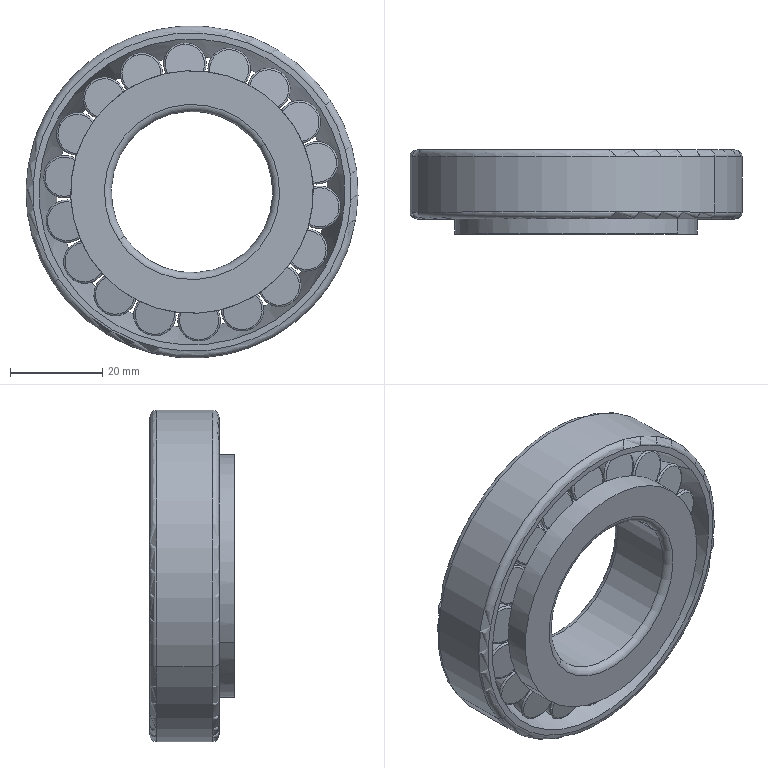Part | NX | features BREP 1 | 1 solid | 172 faces | box 72 x 18.25 x 72 mm | volume 39327 mm3 | torus 80 | cone 44 | plane 40 | cylinder 8 | commonest cylinder face diameters 35 x2 48.163 x2 52.597 x2 72 x2